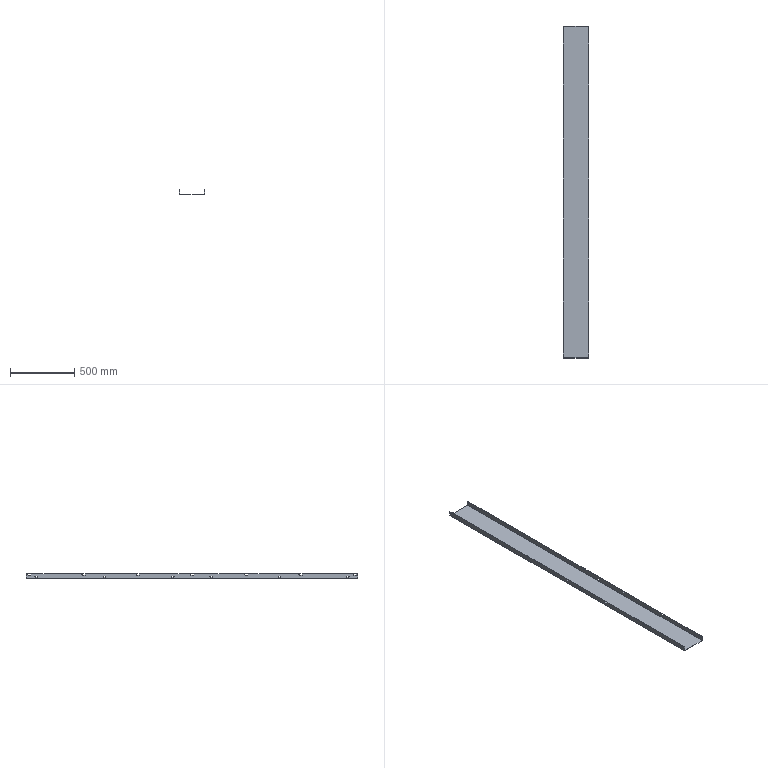Part | 1 solid | 154 faces | box 195 x 2576 x 38.5 mm | volume 825540 mm3 | plane 112 | cylinder 42 | commonest cylinder face diameters 6.4 x24 8.5 x14 0.4 x2 2.8 x2